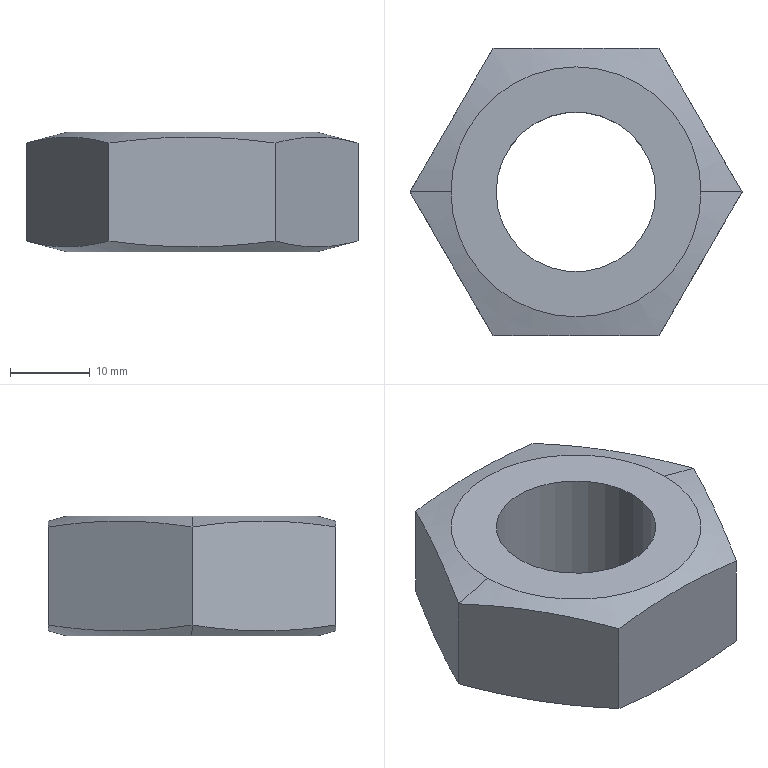Part | SolidWorks | features Extrusion 1, RevCut 1 | 1 solid | 14 faces | box 41.569 x 36 x 15 mm | volume 11785 mm3 | plane 8 | cone 4 | cylinder 2 | commonest cylinder face diameters 20 x2
STEP:
#1=CARTESIAN_POINT('',(-15.651,0.,0.));
#2=VERTEX_POINT('',#1);
#3=CARTESIAN_POINT('',(15.651,0.,0.));
#4=VERTEX_POINT('',#3);
#5=CARTESIAN_POINT('',(0.,0.,0.));
#6=DIRECTION('',(0.,0.,-1.));
#7=DIRECTION('',(1.,0.,0.));
#8=AXIS2_PLACEMENT_3D('',#5,#6,#7);
#9=CIRCLE('',#8,15.651);
#10=EDGE_CURVE('',#2,#4,#9,.T.);
#11=ORIENTED_EDGE('',*,*,#10,.F.);
#12=CARTESIAN_POINT('',(-20.785,0.,1.376));
#13=VERTEX_POINT('',#12);
#14=CARTESIAN_POINT('',(-13.785,0.,-0.5));
#15=DIRECTION('',(-0.9659,0.,0.2588));
#16=VECTOR('',#15,1000.);
#17=LINE('',#14,#16);
#18=EDGE_CURVE('',#2,#13,#17,.T.);
#19=ORIENTED_EDGE('',*,*,#18,.T.);
#20=CARTESIAN_POINT('',(-10.392,18.,1.376));
#21=VERTEX_POINT('',#20);
#22=CARTESIAN_POINT('',(-10.392,18.,1.376));
#23=CARTESIAN_POINT('',(-11.258,16.5,1.144));
#24=CARTESIAN_POINT('',(-12.124,15.,0.9552));
#25=CARTESIAN_POINT('',(-13.856,12.,0.6977));
#26=CARTESIAN_POINT('',(-15.588,9.,0.5613));
#27=CARTESIAN_POINT('',(-17.321,6.,0.6977));
#28=CARTESIAN_POINT('',(-19.053,3.,0.9552));
#29=CARTESIAN_POINT('',(-19.919,1.5,1.144));
#30=CARTESIAN_POINT('',(-20.785,0.,1.376));
#31=B_SPLINE_CURVE_WITH_KNOTS('',3,(#22,#23,#24,#25,#26,#27,#28,#29,#30),.UNSPECIFIED.,.F.,.F.,(4,2,1,2,4),(0.000000231,0.005196,0.01039,0.01559,0.02078),.UNSPECIFIED.);
#32=EDGE_CURVE('',#21,#13,#31,.T.);
#33=ORIENTED_EDGE('',*,*,#32,.F.);
#34=CARTESIAN_POINT('',(10.392,18.,1.376));
#35=VERTEX_POINT('',#34);
#36=CARTESIAN_POINT('',(10.392,18.,1.376));
#37=CARTESIAN_POINT('',(8.685,18.,1.147));
#38=CARTESIAN_POINT('',(6.973,18.,0.9598));
#39=CARTESIAN_POINT('',(3.534,18.,0.7017));
#40=CARTESIAN_POINT('',(1.807,18.,0.6314));
#41=CARTESIAN_POINT('',(-1.664,18.,0.6277));
#42=CARTESIAN_POINT('',(-3.409,18.,0.6944));
#43=CARTESIAN_POINT('',(-6.913,18.,0.9533));
#44=CARTESIAN_POINT('',(-8.657,18.,1.143));
#45=CARTESIAN_POINT('',(-10.392,18.,1.376));
#46=B_SPLINE_CURVE_WITH_KNOTS('',3,(#36,#37,#38,#39,#40,#41,#42,#43,#44,#45),.UNSPECIFIED.,.F.,.F.,(4,2,2,2,4),(0.02131,0.02648,0.03165,0.03681,0.04198),.UNSPECIFIED.);
#47=EDGE_CURVE('',#35,#21,#46,.T.);
#48=ORIENTED_EDGE('',*,*,#47,.F.);
#49=CARTESIAN_POINT('',(20.785,0.,1.376));
#50=VERTEX_POINT('',#49);
#51=CARTESIAN_POINT('',(20.785,0.,1.376));
#52=CARTESIAN_POINT('',(19.919,1.5,1.144));
#53=CARTESIAN_POINT('',(19.053,3.,0.9552));
#54=CARTESIAN_POINT('',(17.321,6.,0.6977));
#55=CARTESIAN_POINT('',(15.588,9.,0.5613));
#56=CARTESIAN_POINT('',(13.856,12.,0.6977));
#57=CARTESIAN_POINT('',(12.124,15.,0.9552));
#58=CARTESIAN_POINT('',(11.258,16.5,1.144));
#59=CARTESIAN_POINT('',(10.392,18.,1.376));
#60=B_SPLINE_CURVE_WITH_KNOTS('',3,(#51,#52,#53,#54,#55,#56,#57,#58,#59),.UNSPECIFIED.,.F.,.F.,(4,2,1,2,4),(0.000000231,0.005196,0.01039,0.01559,0.02078),.UNSPECIFIED.);
#61=EDGE_CURVE('',#50,#35,#60,.T.);
#62=ORIENTED_EDGE('',*,*,#61,.F.);
#63=CARTESIAN_POINT('',(13.785,0.,-0.5));
#64=DIRECTION('',(0.9659,0.,0.2588));
#65=VECTOR('',#64,1000.);
#66=LINE('',#63,#65);
#67=EDGE_CURVE('',#4,#50,#66,.T.);
#68=ORIENTED_EDGE('',*,*,#67,.F.);
#69=EDGE_LOOP('',(#11,#19,#33,#48,#62,#68));
#70=FACE_OUTER_BOUND('',#69,.T.);
#71=CARTESIAN_POINT('',(0.,0.,-0.5));
#72=DIRECTION('',(0.,0.,1.));
#73=DIRECTION('',(1.,0.,0.));
#74=AXIS2_PLACEMENT_3D('',#71,#72,#73);
#75=CONICAL_SURFACE('',#74,13.785,1.309);
#76=ADVANCED_FACE('',(#70),#75,.T.);
#77=CARTESIAN_POINT('',(-15.651,0.,15.));
#78=VERTEX_POINT('',#77);
#79=CARTESIAN_POINT('',(15.651,0.,15.));
#80=VERTEX_POINT('',#79);
#81=CARTESIAN_POINT('',(0.,0.,15.));
#82=DIRECTION('',(0.,0.,-1.));
#83=DIRECTION('',(1.,0.,0.));
#84=AXIS2_PLACEMENT_3D('',#81,#82,#83);
#85=CIRCLE('',#84,15.651);
#86=EDGE_CURVE('',#78,#80,#85,.T.);
#87=ORIENTED_EDGE('',*,*,#86,.T.);
#88=CARTESIAN_POINT('',(20.785,0.,13.624));
#89=VERTEX_POINT('',#88);
#90=CARTESIAN_POINT('',(25.785,0.,12.285));
#91=DIRECTION('',(0.9659,0.,-0.2588));
#92=VECTOR('',#91,1000.);
#93=LINE('',#90,#92);
#94=EDGE_CURVE('',#80,#89,#93,.T.);
#95=ORIENTED_EDGE('',*,*,#94,.T.);
#96=CARTESIAN_POINT('',(10.392,18.,13.624));
#97=VERTEX_POINT('',#96);
#98=CARTESIAN_POINT('',(10.392,18.,13.624));
#99=CARTESIAN_POINT('',(11.258,16.5,13.856));
#100=CARTESIAN_POINT('',(12.124,15.,14.045));
#101=CARTESIAN_POINT('',(13.856,12.,14.302));
#102=CARTESIAN_POINT('',(15.588,9.,14.439));
#103=CARTESIAN_POINT('',(17.321,6.,14.302));
#104=CARTESIAN_POINT('',(19.053,3.,14.045));
#105=CARTESIAN_POINT('',(19.919,1.5,13.856));
#106=CARTESIAN_POINT('',(20.785,0.,13.624));
#107=B_SPLINE_CURVE_WITH_KNOTS('',3,(#98,#99,#100,#101,#102,#103,#104,#105,#106),.UNSPECIFIED.,.F.,.F.,(4,2,1,2,4),(0.000000231,0.005196,0.01039,0.01559,0.02078),.UNSPECIFIED.);
#108=EDGE_CURVE('',#97,#89,#107,.T.);
#109=ORIENTED_EDGE('',*,*,#108,.F.);
#110=CARTESIAN_POINT('',(-10.392,18.,13.624));
#111=VERTEX_POINT('',#110);
#112=CARTESIAN_POINT('',(-10.392,18.,13.624));
#113=CARTESIAN_POINT('',(-8.685,18.,13.853));
#114=CARTESIAN_POINT('',(-6.973,18.,14.04));
#115=CARTESIAN_POINT('',(-3.534,18.,14.298));
#116=CARTESIAN_POINT('',(-1.807,18.,14.369));
#117=CARTESIAN_POINT('',(1.664,18.,14.372));
#118=CARTESIAN_POINT('',(3.409,18.,14.306));
#119=CARTESIAN_POINT('',(6.913,18.,14.047));
#120=CARTESIAN_POINT('',(8.657,18.,13.857));
#121=CARTESIAN_POINT('',(10.392,18.,13.624));
#122=B_SPLINE_CURVE_WITH_KNOTS('',3,(#112,#113,#114,#115,#116,#117,#118,#119,#120,#121),.UNSPECIFIED.,.F.,.F.,(4,2,2,2,4),(0.02131,0.02648,0.03165,0.03681,0.04198),.UNSPECIFIED.);
#123=EDGE_CURVE('',#111,#97,#122,.T.);
#124=ORIENTED_EDGE('',*,*,#123,.F.);
#125=CARTESIAN_POINT('',(-20.785,0.,13.624));
#126=VERTEX_POINT('',#125);
#127=CARTESIAN_POINT('',(-20.785,0.,13.624));
#128=CARTESIAN_POINT('',(-19.919,1.5,13.856));
#129=CARTESIAN_POINT('',(-19.053,3.,14.045));
#130=CARTESIAN_POINT('',(-17.321,6.,14.302));
#131=CARTESIAN_POINT('',(-15.588,9.,14.439));
#132=CARTESIAN_POINT('',(-13.856,12.,14.302));
#133=CARTESIAN_POINT('',(-12.124,15.,14.045));
#134=CARTESIAN_POINT('',(-11.258,16.5,13.856));
#135=CARTESIAN_POINT('',(-10.392,18.,13.624));
#136=B_SPLINE_CURVE_WITH_KNOTS('',3,(#127,#128,#129,#130,#131,#132,#133,#134,#135),.UNSPECIFIED.,.F.,.F.,(4,2,1,2,4),(0.000000231,0.005196,0.01039,0.01559,0.02078),.UNSPECIFIED.);
#137=EDGE_CURVE('',#126,#111,#136,.T.);
#138=ORIENTED_EDGE('',*,*,#137,.F.);
#139=CARTESIAN_POINT('',(-25.785,0.,12.285));
#140=DIRECTION('',(-0.9659,0.,-0.2588));
#141=VECTOR('',#140,1000.);
#142=LINE('',#139,#141);
#143=EDGE_CURVE('',#78,#126,#142,.T.);
#144=ORIENTED_EDGE('',*,*,#143,.F.);
#145=EDGE_LOOP('',(#87,#95,#109,#124,#138,#144));
#146=FACE_OUTER_BOUND('',#145,.T.);
#147=CARTESIAN_POINT('',(0.,0.,12.285));
#148=DIRECTION('',(0.,0.,-1.));
#149=DIRECTION('',(-1.,0.,0.));
#150=AXIS2_PLACEMENT_3D('',#147,#148,#149);
#151=CONICAL_SURFACE('',#150,25.785,1.309);
#152=ADVANCED_FACE('',(#146),#151,.T.);
#153=CARTESIAN_POINT('',(-10.,0.,15.));
#154=VERTEX_POINT('',#153);
#155=CARTESIAN_POINT('',(10.,0.,15.));
#156=VERTEX_POINT('',#155);
#157=CARTESIAN_POINT('',(0.,0.,15.));
#158=DIRECTION('',(0.,0.,1.));
#159=DIRECTION('',(1.,0.,0.));
#160=AXIS2_PLACEMENT_3D('',#157,#158,#159);
#161=CIRCLE('',#160,10.);
#162=EDGE_CURVE('',#154,#156,#161,.T.);
#163=ORIENTED_EDGE('',*,*,#162,.T.);
#164=CARTESIAN_POINT('',(10.,0.,0.));
#165=VERTEX_POINT('',#164);
#166=CARTESIAN_POINT('',(10.,0.,15.));
#167=DIRECTION('',(0.,0.,-1.));
#168=VECTOR('',#167,1000.);
#169=LINE('',#166,#168);
#170=EDGE_CURVE('',#156,#165,#169,.T.);
#171=ORIENTED_EDGE('',*,*,#170,.T.);
#172=CARTESIAN_POINT('',(-10.,0.,0.));
#173=VERTEX_POINT('',#172);
#174=CARTESIAN_POINT('',(0.,0.,0.));
#175=DIRECTION('',(0.,0.,1.));
#176=DIRECTION('',(1.,0.,0.));
#177=AXIS2_PLACEMENT_3D('',#174,#175,#176);
#178=CIRCLE('',#177,10.);
#179=EDGE_CURVE('',#173,#165,#178,.T.);
#180=ORIENTED_EDGE('',*,*,#179,.F.);
#181=CARTESIAN_POINT('',(-10.,0.,15.));
#182=DIRECTION('',(0.,0.,-1.));
#183=VECTOR('',#182,1000.);
#184=LINE('',#181,#183);
#185=EDGE_CURVE('',#154,#173,#184,.T.);
#186=ORIENTED_EDGE('',*,*,#185,.F.);
#187=EDGE_LOOP('',(#163,#171,#180,#186));
#188=FACE_OUTER_BOUND('',#187,.T.);
#189=CARTESIAN_POINT('',(0.,0.,15.));
#190=DIRECTION('',(0.,0.,-1.));
#191=DIRECTION('',(-1.,0.,0.));
#192=AXIS2_PLACEMENT_3D('',#189,#190,#191);
#193=CYLINDRICAL_SURFACE('',#192,10.);
#194=ADVANCED_FACE('',(#188),#193,.F.);
#195=ORIENTED_EDGE('',*,*,#162,.F.);
#196=CARTESIAN_POINT('',(0.,0.,15.));
#197=DIRECTION('',(0.,0.,1.));
#198=DIRECTION('',(1.,0.,0.));
#199=AXIS2_PLACEMENT_3D('',#196,#197,#198);
#200=CIRCLE('',#199,10.);
#201=EDGE_CURVE('',#156,#154,#200,.T.);
#202=ORIENTED_EDGE('',*,*,#201,.F.);
#203=EDGE_LOOP('',(#195,#202));
#204=FACE_BOUND('',#203,.T.);
#205=ORIENTED_EDGE('',*,*,#86,.F.);
#206=CARTESIAN_POINT('',(0.,0.,15.));
#207=DIRECTION('',(0.,0.,-1.));
#208=DIRECTION('',(1.,0.,0.));
#209=AXIS2_PLACEMENT_3D('',#206,#207,#208);
#210=CIRCLE('',#209,15.651);
#211=EDGE_CURVE('',#80,#78,#210,.T.);
#212=ORIENTED_EDGE('',*,*,#211,.F.);
#213=EDGE_LOOP('',(#205,#212));
#214=FACE_OUTER_BOUND('',#213,.T.);
#215=CARTESIAN_POINT('',(0.,0.,15.));
#216=DIRECTION('',(0.,0.,1.));
#217=DIRECTION('',(1.,0.,0.));
#218=AXIS2_PLACEMENT_3D('',#215,#216,#217);
#219=PLANE('',#218);
#220=ADVANCED_FACE('',(#204,#214),#219,.T.);
#221=ORIENTED_EDGE('',*,*,#179,.T.);
#222=CARTESIAN_POINT('',(0.,0.,0.));
#223=DIRECTION('',(0.,0.,1.));
#224=DIRECTION('',(1.,0.,0.));
#225=AXIS2_PLACEMENT_3D('',#222,#223,#224);
#226=CIRCLE('',#225,10.);
#227=EDGE_CURVE('',#165,#173,#226,.T.);
#228=ORIENTED_EDGE('',*,*,#227,.T.);
#229=EDGE_LOOP('',(#221,#228));
#230=FACE_BOUND('',#229,.T.);
#231=CARTESIAN_POINT('',(0.,0.,0.));
#232=DIRECTION('',(0.,0.,-1.));
#233=DIRECTION('',(1.,0.,0.));
#234=AXIS2_PLACEMENT_3D('',#231,#232,#233);
#235=CIRCLE('',#234,15.651);
#236=EDGE_CURVE('',#4,#2,#235,.T.);
#237=ORIENTED_EDGE('',*,*,#236,.T.);
#238=ORIENTED_EDGE('',*,*,#10,.T.);
#239=EDGE_LOOP('',(#237,#238));
#240=FACE_OUTER_BOUND('',#239,.T.);
#241=CARTESIAN_POINT('',(0.,0.,0.));
#242=DIRECTION('',(0.,0.,1.));
#243=DIRECTION('',(1.,0.,0.));
#244=AXIS2_PLACEMENT_3D('',#241,#242,#243);
#245=PLANE('',#244);
#246=ADVANCED_FACE('',(#230,#240),#245,.F.);
#247=ORIENTED_EDGE('',*,*,#170,.F.);
#248=ORIENTED_EDGE('',*,*,#201,.T.);
#249=ORIENTED_EDGE('',*,*,#185,.T.);
#250=ORIENTED_EDGE('',*,*,#227,.F.);
#251=EDGE_LOOP('',(#247,#248,#249,#250));
#252=FACE_OUTER_BOUND('',#251,.T.);
#253=CARTESIAN_POINT('',(0.,0.,15.));
#254=DIRECTION('',(0.,0.,-1.));
#255=DIRECTION('',(-1.,0.,0.));
#256=AXIS2_PLACEMENT_3D('',#253,#254,#255);
#257=CYLINDRICAL_SURFACE('',#256,10.);
#258=ADVANCED_FACE('',(#252),#257,.F.);
#259=ORIENTED_EDGE('',*,*,#94,.F.);
#260=ORIENTED_EDGE('',*,*,#211,.T.);
#261=ORIENTED_EDGE('',*,*,#143,.T.);
#262=CARTESIAN_POINT('',(-10.392,-18.,13.624));
#263=VERTEX_POINT('',#262);
#264=CARTESIAN_POINT('',(-10.392,-18.,13.624));
#265=CARTESIAN_POINT('',(-11.258,-16.5,13.856));
#266=CARTESIAN_POINT('',(-12.124,-15.,14.045));
#267=CARTESIAN_POINT('',(-13.856,-12.,14.302));
#268=CARTESIAN_POINT('',(-15.588,-9.,14.439));
#269=CARTESIAN_POINT('',(-17.321,-6.,14.302));
#270=CARTESIAN_POINT('',(-19.053,-3.,14.045));
#271=CARTESIAN_POINT('',(-19.919,-1.5,13.856));
#272=CARTESIAN_POINT('',(-20.785,0.,13.624));
#273=B_SPLINE_CURVE_WITH_KNOTS('',3,(#264,#265,#266,#267,#268,#269,#270,#271,#272),.UNSPECIFIED.,.F.,.F.,(4,2,1,2,4),(0.000000231,0.005196,0.01039,0.01559,0.02078),.UNSPECIFIED.);
#274=EDGE_CURVE('',#263,#126,#273,.T.);
#275=ORIENTED_EDGE('',*,*,#274,.F.);
#276=CARTESIAN_POINT('',(10.392,-18.,13.624));
#277=VERTEX_POINT('',#276);
#278=CARTESIAN_POINT('',(10.392,-18.,13.624));
#279=CARTESIAN_POINT('',(8.685,-18.,13.853));
#280=CARTESIAN_POINT('',(6.973,-18.,14.04));
#281=CARTESIAN_POINT('',(3.534,-18.,14.298));
#282=CARTESIAN_POINT('',(1.807,-18.,14.369));
#283=CARTESIAN_POINT('',(-1.664,-18.,14.372));
#284=CARTESIAN_POINT('',(-3.409,-18.,14.306));
#285=CARTESIAN_POINT('',(-6.913,-18.,14.047));
#286=CARTESIAN_POINT('',(-8.657,-18.,13.857));
#287=CARTESIAN_POINT('',(-10.392,-18.,13.624));
#288=B_SPLINE_CURVE_WITH_KNOTS('',3,(#278,#279,#280,#281,#282,#283,#284,#285,#286,#287),.UNSPECIFIED.,.F.,.F.,(4,2,2,2,4),(0.02131,0.02648,0.03165,0.03681,0.04198),.UNSPECIFIED.);
#289=EDGE_CURVE('',#277,#263,#288,.T.);
#290=ORIENTED_EDGE('',*,*,#289,.F.);
#291=CARTESIAN_POINT('',(20.785,0.,13.624));
#292=CARTESIAN_POINT('',(19.919,-1.5,13.856));
#293=CARTESIAN_POINT('',(19.053,-3.,14.045));
#294=CARTESIAN_POINT('',(17.321,-6.,14.302));
#295=CARTESIAN_POINT('',(15.588,-9.,14.439));
#296=CARTESIAN_POINT('',(13.856,-12.,14.302));
#297=CARTESIAN_POINT('',(12.124,-15.,14.045));
#298=CARTESIAN_POINT('',(11.258,-16.5,13.856));
#299=CARTESIAN_POINT('',(10.392,-18.,13.624));
#300=B_SPLINE_CURVE_WITH_KNOTS('',3,(#291,#292,#293,#294,#295,#296,#297,#298,#299),.UNSPECIFIED.,.F.,.F.,(4,2,1,2,4),(0.000000231,0.005196,0.01039,0.01559,0.02078),.UNSPECIFIED.);
#301=EDGE_CURVE('',#89,#277,#300,.T.);
#302=ORIENTED_EDGE('',*,*,#301,.F.);
#303=EDGE_LOOP('',(#259,#260,#261,#275,#290,#302));
#304=FACE_OUTER_BOUND('',#303,.T.);
#305=CARTESIAN_POINT('',(0.,0.,12.285));
#306=DIRECTION('',(0.,0.,-1.));
#307=DIRECTION('',(-1.,0.,0.));
#308=AXIS2_PLACEMENT_3D('',#305,#306,#307);
#309=CONICAL_SURFACE('',#308,25.785,1.309);
#310=ADVANCED_FACE('',(#304),#309,.T.);
#311=ORIENTED_EDGE('',*,*,#18,.F.);
#312=ORIENTED_EDGE('',*,*,#236,.F.);
#313=ORIENTED_EDGE('',*,*,#67,.T.);
#314=CARTESIAN_POINT('',(10.392,-18.,1.376));
#315=VERTEX_POINT('',#314);
#316=CARTESIAN_POINT('',(10.392,-18.,1.376));
#317=CARTESIAN_POINT('',(11.258,-16.5,1.144));
#318=CARTESIAN_POINT('',(12.124,-15.,0.9552));
#319=CARTESIAN_POINT('',(13.856,-12.,0.6977));
#320=CARTESIAN_POINT('',(15.588,-9.,0.5613));
#321=CARTESIAN_POINT('',(17.321,-6.,0.6977));
#322=CARTESIAN_POINT('',(19.053,-3.,0.9552));
#323=CARTESIAN_POINT('',(19.919,-1.5,1.144));
#324=CARTESIAN_POINT('',(20.785,0.,1.376));
#325=B_SPLINE_CURVE_WITH_KNOTS('',3,(#316,#317,#318,#319,#320,#321,#322,#323,#324),.UNSPECIFIED.,.F.,.F.,(4,2,1,2,4),(0.000000231,0.005196,0.01039,0.01559,0.02078),.UNSPECIFIED.);
#326=EDGE_CURVE('',#315,#50,#325,.T.);
#327=ORIENTED_EDGE('',*,*,#326,.F.);
#328=CARTESIAN_POINT('',(-10.392,-18.,1.376));
#329=VERTEX_POINT('',#328);
#330=CARTESIAN_POINT('',(-10.392,-18.,1.376));
#331=CARTESIAN_POINT('',(-8.685,-18.,1.147));
#332=CARTESIAN_POINT('',(-6.973,-18.,0.9598));
#333=CARTESIAN_POINT('',(-3.534,-18.,0.7017));
#334=CARTESIAN_POINT('',(-1.807,-18.,0.6314));
#335=CARTESIAN_POINT('',(1.664,-18.,0.6277));
#336=CARTESIAN_POINT('',(3.409,-18.,0.6944));
#337=CARTESIAN_POINT('',(6.913,-18.,0.9533));
#338=CARTESIAN_POINT('',(8.657,-18.,1.143));
#339=CARTESIAN_POINT('',(10.392,-18.,1.376));
#340=B_SPLINE_CURVE_WITH_KNOTS('',3,(#330,#331,#332,#333,#334,#335,#336,#337,#338,#339),.UNSPECIFIED.,.F.,.F.,(4,2,2,2,4),(0.02131,0.02648,0.03165,0.03681,0.04198),.UNSPECIFIED.);
#341=EDGE_CURVE('',#329,#315,#340,.T.);
#342=ORIENTED_EDGE('',*,*,#341,.F.);
#343=CARTESIAN_POINT('',(-20.785,0.,1.376));
#344=CARTESIAN_POINT('',(-19.919,-1.5,1.144));
#345=CARTESIAN_POINT('',(-19.053,-3.,0.9552));
#346=CARTESIAN_POINT('',(-17.321,-6.,0.6977));
#347=CARTESIAN_POINT('',(-15.588,-9.,0.5613));
#348=CARTESIAN_POINT('',(-13.856,-12.,0.6977));
#349=CARTESIAN_POINT('',(-12.124,-15.,0.9552));
#350=CARTESIAN_POINT('',(-11.258,-16.5,1.144));
#351=CARTESIAN_POINT('',(-10.392,-18.,1.376));
#352=B_SPLINE_CURVE_WITH_KNOTS('',3,(#343,#344,#345,#346,#347,#348,#349,#350,#351),.UNSPECIFIED.,.F.,.F.,(4,2,1,2,4),(0.000000231,0.005196,0.01039,0.01559,0.02078),.UNSPECIFIED.);
#353=EDGE_CURVE('',#13,#329,#352,.T.);
#354=ORIENTED_EDGE('',*,*,#353,.F.);
#355=EDGE_LOOP('',(#311,#312,#313,#327,#342,#354));
#356=FACE_OUTER_BOUND('',#355,.T.);
#357=CARTESIAN_POINT('',(0.,0.,-0.5));
#358=DIRECTION('',(0.,0.,1.));
#359=DIRECTION('',(1.,0.,0.));
#360=AXIS2_PLACEMENT_3D('',#357,#358,#359);
#361=CONICAL_SURFACE('',#360,13.785,1.309);
#362=ADVANCED_FACE('',(#356),#361,.T.);
#363=CARTESIAN_POINT('',(10.392,18.,15.));
#364=DIRECTION('',(0.,0.,-1.));
#365=VECTOR('',#364,1000.);
#366=LINE('',#363,#365);
#367=EDGE_CURVE('',#97,#35,#366,.T.);
#368=ORIENTED_EDGE('',*,*,#367,.T.);
#369=ORIENTED_EDGE('',*,*,#47,.T.);
#370=CARTESIAN_POINT('',(-10.392,18.,15.));
#371=DIRECTION('',(0.,0.,-1.));
#372=VECTOR('',#371,1000.);
#373=LINE('',#370,#372);
#374=EDGE_CURVE('',#111,#21,#373,.T.);
#375=ORIENTED_EDGE('',*,*,#374,.F.);
#376=ORIENTED_EDGE('',*,*,#123,.T.);
#377=EDGE_LOOP('',(#368,#369,#375,#376));
#378=FACE_OUTER_BOUND('',#377,.T.);
#379=CARTESIAN_POINT('',(10.392,18.,15.));
#380=DIRECTION('',(0.,-1.,0.));
#381=DIRECTION('',(0.,0.,-1.));
#382=AXIS2_PLACEMENT_3D('',#379,#380,#381);
#383=PLANE('',#382);
#384=ADVANCED_FACE('',(#378),#383,.F.);
#385=CARTESIAN_POINT('',(20.785,0.,15.));
#386=DIRECTION('',(0.,0.,-1.));
#387=VECTOR('',#386,1000.);
#388=LINE('',#385,#387);
#389=EDGE_CURVE('',#89,#50,#388,.T.);
#390=ORIENTED_EDGE('',*,*,#389,.T.);
#391=ORIENTED_EDGE('',*,*,#61,.T.);
#392=ORIENTED_EDGE('',*,*,#367,.F.);
#393=ORIENTED_EDGE('',*,*,#108,.T.);
#394=EDGE_LOOP('',(#390,#391,#392,#393));
#395=FACE_OUTER_BOUND('',#394,.T.);
#396=CARTESIAN_POINT('',(20.785,0.,15.));
#397=DIRECTION('',(-0.866,-0.5,0.));
#398=DIRECTION('',(0.5,-0.866,0.));
#399=AXIS2_PLACEMENT_3D('',#396,#397,#398);
#400=PLANE('',#399);
#401=ADVANCED_FACE('',(#395),#400,.F.);
#402=CARTESIAN_POINT('',(10.392,-18.,15.));
#403=DIRECTION('',(0.,0.,-1.));
#404=VECTOR('',#403,1000.);
#405=LINE('',#402,#404);
#406=EDGE_CURVE('',#277,#315,#405,.T.);
#407=ORIENTED_EDGE('',*,*,#406,.T.);
#408=ORIENTED_EDGE('',*,*,#326,.T.);
#409=ORIENTED_EDGE('',*,*,#389,.F.);
#410=ORIENTED_EDGE('',*,*,#301,.T.);
#411=EDGE_LOOP('',(#407,#408,#409,#410));
#412=FACE_OUTER_BOUND('',#411,.T.);
#413=CARTESIAN_POINT('',(10.392,-18.,15.));
#414=DIRECTION('',(-0.866,0.5,0.));
#415=DIRECTION('',(-0.5,-0.866,0.));
#416=AXIS2_PLACEMENT_3D('',#413,#414,#415);
#417=PLANE('',#416);
#418=ADVANCED_FACE('',(#412),#417,.F.);
#419=CARTESIAN_POINT('',(-10.392,-18.,15.));
#420=DIRECTION('',(0.,0.,-1.));
#421=VECTOR('',#420,1000.);
#422=LINE('',#419,#421);
#423=EDGE_CURVE('',#263,#329,#422,.T.);
#424=ORIENTED_EDGE('',*,*,#423,.T.);
#425=ORIENTED_EDGE('',*,*,#341,.T.);
#426=ORIENTED_EDGE('',*,*,#406,.F.);
#427=ORIENTED_EDGE('',*,*,#289,.T.);
#428=EDGE_LOOP('',(#424,#425,#426,#427));
#429=FACE_OUTER_BOUND('',#428,.T.);
#430=CARTESIAN_POINT('',(-10.392,-18.,15.));
#431=DIRECTION('',(0.,1.,0.));
#432=DIRECTION('',(-1.,0.,0.));
#433=AXIS2_PLACEMENT_3D('',#430,#431,#432);
#434=PLANE('',#433);
#435=ADVANCED_FACE('',(#429),#434,.F.);
#436=CARTESIAN_POINT('',(-20.785,0.,15.));
#437=DIRECTION('',(0.,0.,-1.));
#438=VECTOR('',#437,1000.);
#439=LINE('',#436,#438);
#440=EDGE_CURVE('',#126,#13,#439,.T.);
#441=ORIENTED_EDGE('',*,*,#440,.T.);
#442=ORIENTED_EDGE('',*,*,#353,.T.);
#443=ORIENTED_EDGE('',*,*,#423,.F.);
#444=ORIENTED_EDGE('',*,*,#274,.T.);
#445=EDGE_LOOP('',(#441,#442,#443,#444));
#446=FACE_OUTER_BOUND('',#445,.T.);
#447=CARTESIAN_POINT('',(-20.785,0.,15.));
#448=DIRECTION('',(0.866,0.5,0.));
#449=DIRECTION('',(-0.5,0.866,0.));
#450=AXIS2_PLACEMENT_3D('',#447,#448,#449);
#451=PLANE('',#450);
#452=ADVANCED_FACE('',(#446),#451,.F.);
#453=ORIENTED_EDGE('',*,*,#374,.T.);
#454=ORIENTED_EDGE('',*,*,#32,.T.);
#455=ORIENTED_EDGE('',*,*,#440,.F.);
#456=ORIENTED_EDGE('',*,*,#137,.T.);
#457=EDGE_LOOP('',(#453,#454,#455,#456));
#458=FACE_OUTER_BOUND('',#457,.T.);
#459=CARTESIAN_POINT('',(-10.392,18.,15.));
#460=DIRECTION('',(0.866,-0.5,0.));
#461=DIRECTION('',(0.5,0.866,0.));
#462=AXIS2_PLACEMENT_3D('',#459,#460,#461);
#463=PLANE('',#462);
#464=ADVANCED_FACE('',(#458),#463,.F.);
#465=CLOSED_SHELL('',(#76,#152,#194,#220,#246,#258,#310,#362,#384,#401,#418,#435,#452,#464));
#466=MANIFOLD_SOLID_BREP('',#465);
#467=CARTESIAN_POINT('',(0.,0.,0.));
#468=DIRECTION('',(0.,0.,1.));
#469=DIRECTION('',(1.,0.,0.));
#470=AXIS2_PLACEMENT_3D('',#467,#468,#469);
#471=(LENGTH_UNIT()NAMED_UNIT(*)SI_UNIT(.MILLI.,.METRE.));
#472=UNCERTAINTY_MEASURE_WITH_UNIT(LENGTH_MEASURE(0.00001),#471,'','');
#473=(NAMED_UNIT(*)PLANE_ANGLE_UNIT()SI_UNIT($,.RADIAN.));
#474=(NAMED_UNIT(*)SI_UNIT($,.STERADIAN.)SOLID_ANGLE_UNIT());
#475=(GEOMETRIC_REPRESENTATION_CONTEXT(3)GLOBAL_UNCERTAINTY_ASSIGNED_CONTEXT((#472))GLOBAL_UNIT_ASSIGNED_CONTEXT((#471,#473,#474))REPRESENTATION_CONTEXT('',''));
#476=ADVANCED_BREP_SHAPE_REPRESENTATION('',(#466,#470),#475);